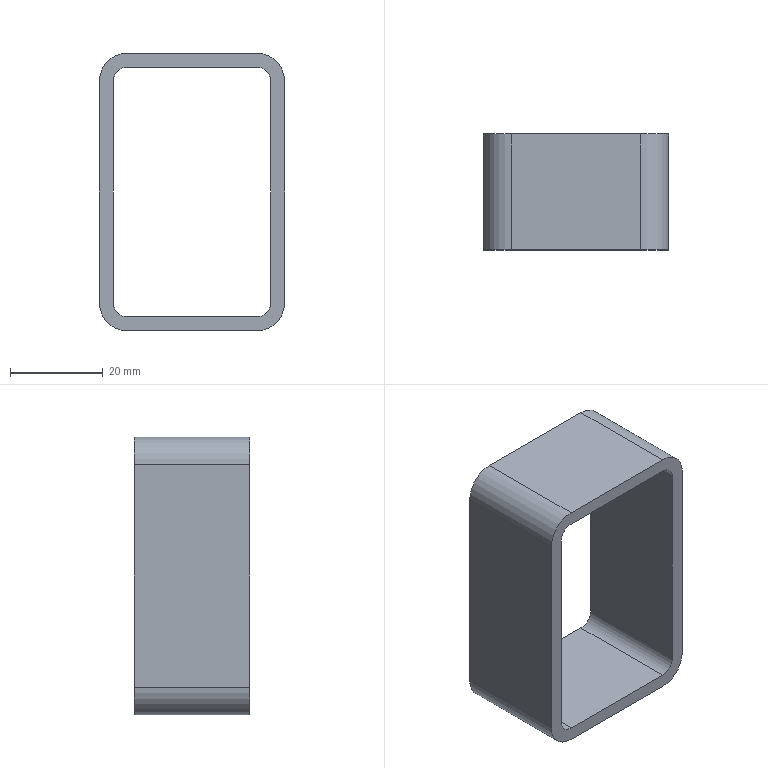Part | SolidWorks | features WeldMemberFeat 1, WeldmentFeature 1 | 1 solid | 18 faces | box 40 x 25 x 60 mm | volume 13521 mm3 | plane 10 | cylinder 8 | commonest cylinder face diameters 6 x4 12 x4
STEP:
#1=CARTESIAN_POINT('',(-20.,0.,24.));
#2=VERTEX_POINT('',#1);
#3=CARTESIAN_POINT('',(-14.,0.,30.));
#4=VERTEX_POINT('',#3);
#5=CARTESIAN_POINT('',(-14.,0.,24.));
#6=DIRECTION('',(0.,1.,0.));
#7=DIRECTION('',(0.,0.,1.));
#8=AXIS2_PLACEMENT_3D('',#5,#6,#7);
#9=CIRCLE('',#8,6.);
#10=EDGE_CURVE('',#2,#4,#9,.T.);
#11=ORIENTED_EDGE('',*,*,#10,.T.);
#12=CARTESIAN_POINT('',(-14.,25.,30.));
#13=VERTEX_POINT('',#12);
#14=CARTESIAN_POINT('',(-14.,25.,30.));
#15=DIRECTION('',(0.,-1.,0.));
#16=VECTOR('',#15,1000.);
#17=LINE('',#14,#16);
#18=EDGE_CURVE('',#13,#4,#17,.T.);
#19=ORIENTED_EDGE('',*,*,#18,.F.);
#20=CARTESIAN_POINT('',(-20.,25.,24.));
#21=VERTEX_POINT('',#20);
#22=CARTESIAN_POINT('',(-14.,25.,24.));
#23=DIRECTION('',(0.,1.,0.));
#24=DIRECTION('',(0.,0.,1.));
#25=AXIS2_PLACEMENT_3D('',#22,#23,#24);
#26=CIRCLE('',#25,6.);
#27=EDGE_CURVE('',#21,#13,#26,.T.);
#28=ORIENTED_EDGE('',*,*,#27,.F.);
#29=CARTESIAN_POINT('',(-20.,25.,24.));
#30=DIRECTION('',(0.,-1.,0.));
#31=VECTOR('',#30,1000.);
#32=LINE('',#29,#31);
#33=EDGE_CURVE('',#21,#2,#32,.T.);
#34=ORIENTED_EDGE('',*,*,#33,.T.);
#35=EDGE_LOOP('',(#11,#19,#28,#34));
#36=FACE_OUTER_BOUND('',#35,.T.);
#37=CARTESIAN_POINT('',(-14.,25.,24.));
#38=DIRECTION('',(0.,-1.,0.));
#39=DIRECTION('',(0.,0.,-1.));
#40=AXIS2_PLACEMENT_3D('',#37,#38,#39);
#41=CYLINDRICAL_SURFACE('',#40,6.);
#42=ADVANCED_FACE('',(#36),#41,.T.);
#43=CARTESIAN_POINT('',(14.,0.,30.));
#44=VERTEX_POINT('',#43);
#45=CARTESIAN_POINT('',(-14.,0.,30.));
#46=DIRECTION('',(1.,0.,0.));
#47=VECTOR('',#46,1000.);
#48=LINE('',#45,#47);
#49=EDGE_CURVE('',#4,#44,#48,.T.);
#50=ORIENTED_EDGE('',*,*,#49,.T.);
#51=CARTESIAN_POINT('',(14.,25.,30.));
#52=VERTEX_POINT('',#51);
#53=CARTESIAN_POINT('',(14.,25.,30.));
#54=DIRECTION('',(0.,-1.,0.));
#55=VECTOR('',#54,1000.);
#56=LINE('',#53,#55);
#57=EDGE_CURVE('',#52,#44,#56,.T.);
#58=ORIENTED_EDGE('',*,*,#57,.F.);
#59=CARTESIAN_POINT('',(-14.,25.,30.));
#60=DIRECTION('',(1.,0.,0.));
#61=VECTOR('',#60,1000.);
#62=LINE('',#59,#61);
#63=EDGE_CURVE('',#13,#52,#62,.T.);
#64=ORIENTED_EDGE('',*,*,#63,.F.);
#65=ORIENTED_EDGE('',*,*,#18,.T.);
#66=EDGE_LOOP('',(#50,#58,#64,#65));
#67=FACE_OUTER_BOUND('',#66,.T.);
#68=CARTESIAN_POINT('',(-14.,25.,30.));
#69=DIRECTION('',(0.,0.,-1.));
#70=DIRECTION('',(-1.,0.,0.));
#71=AXIS2_PLACEMENT_3D('',#68,#69,#70);
#72=PLANE('',#71);
#73=ADVANCED_FACE('',(#67),#72,.F.);
#74=CARTESIAN_POINT('',(20.,0.,24.));
#75=VERTEX_POINT('',#74);
#76=CARTESIAN_POINT('',(14.,0.,24.));
#77=DIRECTION('',(0.,1.,0.));
#78=DIRECTION('',(0.,0.,1.));
#79=AXIS2_PLACEMENT_3D('',#76,#77,#78);
#80=CIRCLE('',#79,6.);
#81=EDGE_CURVE('',#44,#75,#80,.T.);
#82=ORIENTED_EDGE('',*,*,#81,.T.);
#83=CARTESIAN_POINT('',(20.,25.,24.));
#84=VERTEX_POINT('',#83);
#85=CARTESIAN_POINT('',(20.,25.,24.));
#86=DIRECTION('',(0.,-1.,0.));
#87=VECTOR('',#86,1000.);
#88=LINE('',#85,#87);
#89=EDGE_CURVE('',#84,#75,#88,.T.);
#90=ORIENTED_EDGE('',*,*,#89,.F.);
#91=CARTESIAN_POINT('',(14.,25.,24.));
#92=DIRECTION('',(0.,1.,0.));
#93=DIRECTION('',(0.,0.,1.));
#94=AXIS2_PLACEMENT_3D('',#91,#92,#93);
#95=CIRCLE('',#94,6.);
#96=EDGE_CURVE('',#52,#84,#95,.T.);
#97=ORIENTED_EDGE('',*,*,#96,.F.);
#98=ORIENTED_EDGE('',*,*,#57,.T.);
#99=EDGE_LOOP('',(#82,#90,#97,#98));
#100=FACE_OUTER_BOUND('',#99,.T.);
#101=CARTESIAN_POINT('',(14.,25.,24.));
#102=DIRECTION('',(0.,-1.,0.));
#103=DIRECTION('',(0.,0.,-1.));
#104=AXIS2_PLACEMENT_3D('',#101,#102,#103);
#105=CYLINDRICAL_SURFACE('',#104,6.);
#106=ADVANCED_FACE('',(#100),#105,.T.);
#107=CARTESIAN_POINT('',(20.,0.,-24.));
#108=VERTEX_POINT('',#107);
#109=CARTESIAN_POINT('',(20.,0.,-24.));
#110=DIRECTION('',(0.,0.,-1.));
#111=VECTOR('',#110,1000.);
#112=LINE('',#109,#111);
#113=EDGE_CURVE('',#75,#108,#112,.T.);
#114=ORIENTED_EDGE('',*,*,#113,.T.);
#115=CARTESIAN_POINT('',(20.,25.,-24.));
#116=VERTEX_POINT('',#115);
#117=CARTESIAN_POINT('',(20.,25.,-24.));
#118=DIRECTION('',(0.,-1.,0.));
#119=VECTOR('',#118,1000.);
#120=LINE('',#117,#119);
#121=EDGE_CURVE('',#116,#108,#120,.T.);
#122=ORIENTED_EDGE('',*,*,#121,.F.);
#123=CARTESIAN_POINT('',(20.,25.,-24.));
#124=DIRECTION('',(0.,0.,-1.));
#125=VECTOR('',#124,1000.);
#126=LINE('',#123,#125);
#127=EDGE_CURVE('',#84,#116,#126,.T.);
#128=ORIENTED_EDGE('',*,*,#127,.F.);
#129=ORIENTED_EDGE('',*,*,#89,.T.);
#130=EDGE_LOOP('',(#114,#122,#128,#129));
#131=FACE_OUTER_BOUND('',#130,.T.);
#132=CARTESIAN_POINT('',(20.,25.,-24.));
#133=DIRECTION('',(-1.,0.,0.));
#134=DIRECTION('',(0.,0.,1.));
#135=AXIS2_PLACEMENT_3D('',#132,#133,#134);
#136=PLANE('',#135);
#137=ADVANCED_FACE('',(#131),#136,.F.);
#138=CARTESIAN_POINT('',(14.,0.,-30.));
#139=VERTEX_POINT('',#138);
#140=CARTESIAN_POINT('',(14.,0.,-24.));
#141=DIRECTION('',(0.,1.,0.));
#142=DIRECTION('',(0.,0.,1.));
#143=AXIS2_PLACEMENT_3D('',#140,#141,#142);
#144=CIRCLE('',#143,6.);
#145=EDGE_CURVE('',#108,#139,#144,.T.);
#146=ORIENTED_EDGE('',*,*,#145,.T.);
#147=CARTESIAN_POINT('',(14.,25.,-30.));
#148=VERTEX_POINT('',#147);
#149=CARTESIAN_POINT('',(14.,25.,-30.));
#150=DIRECTION('',(0.,-1.,0.));
#151=VECTOR('',#150,1000.);
#152=LINE('',#149,#151);
#153=EDGE_CURVE('',#148,#139,#152,.T.);
#154=ORIENTED_EDGE('',*,*,#153,.F.);
#155=CARTESIAN_POINT('',(14.,25.,-24.));
#156=DIRECTION('',(0.,1.,0.));
#157=DIRECTION('',(0.,0.,1.));
#158=AXIS2_PLACEMENT_3D('',#155,#156,#157);
#159=CIRCLE('',#158,6.);
#160=EDGE_CURVE('',#116,#148,#159,.T.);
#161=ORIENTED_EDGE('',*,*,#160,.F.);
#162=ORIENTED_EDGE('',*,*,#121,.T.);
#163=EDGE_LOOP('',(#146,#154,#161,#162));
#164=FACE_OUTER_BOUND('',#163,.T.);
#165=CARTESIAN_POINT('',(14.,25.,-24.));
#166=DIRECTION('',(0.,-1.,0.));
#167=DIRECTION('',(0.,0.,-1.));
#168=AXIS2_PLACEMENT_3D('',#165,#166,#167);
#169=CYLINDRICAL_SURFACE('',#168,6.);
#170=ADVANCED_FACE('',(#164),#169,.T.);
#171=CARTESIAN_POINT('',(-14.,0.,-30.));
#172=VERTEX_POINT('',#171);
#173=CARTESIAN_POINT('',(14.,0.,-30.));
#174=DIRECTION('',(-1.,0.,0.));
#175=VECTOR('',#174,1000.);
#176=LINE('',#173,#175);
#177=EDGE_CURVE('',#139,#172,#176,.T.);
#178=ORIENTED_EDGE('',*,*,#177,.T.);
#179=CARTESIAN_POINT('',(-14.,25.,-30.));
#180=VERTEX_POINT('',#179);
#181=CARTESIAN_POINT('',(-14.,25.,-30.));
#182=DIRECTION('',(0.,-1.,0.));
#183=VECTOR('',#182,1000.);
#184=LINE('',#181,#183);
#185=EDGE_CURVE('',#180,#172,#184,.T.);
#186=ORIENTED_EDGE('',*,*,#185,.F.);
#187=CARTESIAN_POINT('',(14.,25.,-30.));
#188=DIRECTION('',(-1.,0.,0.));
#189=VECTOR('',#188,1000.);
#190=LINE('',#187,#189);
#191=EDGE_CURVE('',#148,#180,#190,.T.);
#192=ORIENTED_EDGE('',*,*,#191,.F.);
#193=ORIENTED_EDGE('',*,*,#153,.T.);
#194=EDGE_LOOP('',(#178,#186,#192,#193));
#195=FACE_OUTER_BOUND('',#194,.T.);
#196=CARTESIAN_POINT('',(14.,25.,-30.));
#197=DIRECTION('',(0.,0.,1.));
#198=DIRECTION('',(1.,0.,0.));
#199=AXIS2_PLACEMENT_3D('',#196,#197,#198);
#200=PLANE('',#199);
#201=ADVANCED_FACE('',(#195),#200,.F.);
#202=CARTESIAN_POINT('',(-20.,0.,-24.));
#203=VERTEX_POINT('',#202);
#204=CARTESIAN_POINT('',(-14.,0.,-24.));
#205=DIRECTION('',(0.,1.,0.));
#206=DIRECTION('',(0.,0.,1.));
#207=AXIS2_PLACEMENT_3D('',#204,#205,#206);
#208=CIRCLE('',#207,6.);
#209=EDGE_CURVE('',#172,#203,#208,.T.);
#210=ORIENTED_EDGE('',*,*,#209,.T.);
#211=CARTESIAN_POINT('',(-20.,25.,-24.));
#212=VERTEX_POINT('',#211);
#213=CARTESIAN_POINT('',(-20.,25.,-24.));
#214=DIRECTION('',(0.,-1.,0.));
#215=VECTOR('',#214,1000.);
#216=LINE('',#213,#215);
#217=EDGE_CURVE('',#212,#203,#216,.T.);
#218=ORIENTED_EDGE('',*,*,#217,.F.);
#219=CARTESIAN_POINT('',(-14.,25.,-24.));
#220=DIRECTION('',(0.,1.,0.));
#221=DIRECTION('',(0.,0.,1.));
#222=AXIS2_PLACEMENT_3D('',#219,#220,#221);
#223=CIRCLE('',#222,6.);
#224=EDGE_CURVE('',#180,#212,#223,.T.);
#225=ORIENTED_EDGE('',*,*,#224,.F.);
#226=ORIENTED_EDGE('',*,*,#185,.T.);
#227=EDGE_LOOP('',(#210,#218,#225,#226));
#228=FACE_OUTER_BOUND('',#227,.T.);
#229=CARTESIAN_POINT('',(-14.,25.,-24.));
#230=DIRECTION('',(0.,-1.,0.));
#231=DIRECTION('',(0.,0.,-1.));
#232=AXIS2_PLACEMENT_3D('',#229,#230,#231);
#233=CYLINDRICAL_SURFACE('',#232,6.);
#234=ADVANCED_FACE('',(#228),#233,.T.);
#235=CARTESIAN_POINT('',(14.,0.,27.));
#236=VERTEX_POINT('',#235);
#237=CARTESIAN_POINT('',(17.,0.,24.));
#238=VERTEX_POINT('',#237);
#239=CARTESIAN_POINT('',(14.,0.,24.));
#240=DIRECTION('',(0.,1.,0.));
#241=DIRECTION('',(0.,0.,1.));
#242=AXIS2_PLACEMENT_3D('',#239,#240,#241);
#243=CIRCLE('',#242,3.);
#244=EDGE_CURVE('',#236,#238,#243,.T.);
#245=ORIENTED_EDGE('',*,*,#244,.F.);
#246=CARTESIAN_POINT('',(14.,25.,27.));
#247=VERTEX_POINT('',#246);
#248=CARTESIAN_POINT('',(14.,25.,27.));
#249=DIRECTION('',(0.,-1.,0.));
#250=VECTOR('',#249,1000.);
#251=LINE('',#248,#250);
#252=EDGE_CURVE('',#247,#236,#251,.T.);
#253=ORIENTED_EDGE('',*,*,#252,.F.);
#254=CARTESIAN_POINT('',(17.,25.,24.));
#255=VERTEX_POINT('',#254);
#256=CARTESIAN_POINT('',(14.,25.,24.));
#257=DIRECTION('',(0.,1.,0.));
#258=DIRECTION('',(0.,0.,1.));
#259=AXIS2_PLACEMENT_3D('',#256,#257,#258);
#260=CIRCLE('',#259,3.);
#261=EDGE_CURVE('',#247,#255,#260,.T.);
#262=ORIENTED_EDGE('',*,*,#261,.T.);
#263=CARTESIAN_POINT('',(17.,25.,24.));
#264=DIRECTION('',(0.,-1.,0.));
#265=VECTOR('',#264,1000.);
#266=LINE('',#263,#265);
#267=EDGE_CURVE('',#255,#238,#266,.T.);
#268=ORIENTED_EDGE('',*,*,#267,.T.);
#269=EDGE_LOOP('',(#245,#253,#262,#268));
#270=FACE_OUTER_BOUND('',#269,.T.);
#271=CARTESIAN_POINT('',(14.,25.,24.));
#272=DIRECTION('',(0.,-1.,0.));
#273=DIRECTION('',(0.,0.,-1.));
#274=AXIS2_PLACEMENT_3D('',#271,#272,#273);
#275=CYLINDRICAL_SURFACE('',#274,3.);
#276=ADVANCED_FACE('',(#270),#275,.F.);
#277=CARTESIAN_POINT('',(-14.,0.,27.));
#278=VERTEX_POINT('',#277);
#279=CARTESIAN_POINT('',(-14.,0.,27.));
#280=DIRECTION('',(1.,0.,0.));
#281=VECTOR('',#280,1000.);
#282=LINE('',#279,#281);
#283=EDGE_CURVE('',#278,#236,#282,.T.);
#284=ORIENTED_EDGE('',*,*,#283,.F.);
#285=CARTESIAN_POINT('',(-14.,25.,27.));
#286=VERTEX_POINT('',#285);
#287=CARTESIAN_POINT('',(-14.,25.,27.));
#288=DIRECTION('',(0.,-1.,0.));
#289=VECTOR('',#288,1000.);
#290=LINE('',#287,#289);
#291=EDGE_CURVE('',#286,#278,#290,.T.);
#292=ORIENTED_EDGE('',*,*,#291,.F.);
#293=CARTESIAN_POINT('',(-14.,25.,27.));
#294=DIRECTION('',(1.,0.,0.));
#295=VECTOR('',#294,1000.);
#296=LINE('',#293,#295);
#297=EDGE_CURVE('',#286,#247,#296,.T.);
#298=ORIENTED_EDGE('',*,*,#297,.T.);
#299=ORIENTED_EDGE('',*,*,#252,.T.);
#300=EDGE_LOOP('',(#284,#292,#298,#299));
#301=FACE_OUTER_BOUND('',#300,.T.);
#302=CARTESIAN_POINT('',(-14.,25.,27.));
#303=DIRECTION('',(0.,0.,-1.));
#304=DIRECTION('',(-1.,0.,0.));
#305=AXIS2_PLACEMENT_3D('',#302,#303,#304);
#306=PLANE('',#305);
#307=ADVANCED_FACE('',(#301),#306,.T.);
#308=CARTESIAN_POINT('',(-17.,0.,24.));
#309=VERTEX_POINT('',#308);
#310=CARTESIAN_POINT('',(-14.,0.,24.));
#311=DIRECTION('',(0.,1.,0.));
#312=DIRECTION('',(0.,0.,1.));
#313=AXIS2_PLACEMENT_3D('',#310,#311,#312);
#314=CIRCLE('',#313,3.);
#315=EDGE_CURVE('',#309,#278,#314,.T.);
#316=ORIENTED_EDGE('',*,*,#315,.F.);
#317=CARTESIAN_POINT('',(-17.,25.,24.));
#318=VERTEX_POINT('',#317);
#319=CARTESIAN_POINT('',(-17.,25.,24.));
#320=DIRECTION('',(0.,-1.,0.));
#321=VECTOR('',#320,1000.);
#322=LINE('',#319,#321);
#323=EDGE_CURVE('',#318,#309,#322,.T.);
#324=ORIENTED_EDGE('',*,*,#323,.F.);
#325=CARTESIAN_POINT('',(-14.,25.,24.));
#326=DIRECTION('',(0.,1.,0.));
#327=DIRECTION('',(0.,0.,1.));
#328=AXIS2_PLACEMENT_3D('',#325,#326,#327);
#329=CIRCLE('',#328,3.);
#330=EDGE_CURVE('',#318,#286,#329,.T.);
#331=ORIENTED_EDGE('',*,*,#330,.T.);
#332=ORIENTED_EDGE('',*,*,#291,.T.);
#333=EDGE_LOOP('',(#316,#324,#331,#332));
#334=FACE_OUTER_BOUND('',#333,.T.);
#335=CARTESIAN_POINT('',(-14.,25.,24.));
#336=DIRECTION('',(0.,-1.,0.));
#337=DIRECTION('',(0.,0.,-1.));
#338=AXIS2_PLACEMENT_3D('',#335,#336,#337);
#339=CYLINDRICAL_SURFACE('',#338,3.);
#340=ADVANCED_FACE('',(#334),#339,.F.);
#341=CARTESIAN_POINT('',(-17.,0.,-24.));
#342=VERTEX_POINT('',#341);
#343=CARTESIAN_POINT('',(-17.,0.,24.));
#344=DIRECTION('',(0.,0.,1.));
#345=VECTOR('',#344,1000.);
#346=LINE('',#343,#345);
#347=EDGE_CURVE('',#342,#309,#346,.T.);
#348=ORIENTED_EDGE('',*,*,#347,.F.);
#349=CARTESIAN_POINT('',(-17.,25.,-24.));
#350=VERTEX_POINT('',#349);
#351=CARTESIAN_POINT('',(-17.,25.,-24.));
#352=DIRECTION('',(0.,-1.,0.));
#353=VECTOR('',#352,1000.);
#354=LINE('',#351,#353);
#355=EDGE_CURVE('',#350,#342,#354,.T.);
#356=ORIENTED_EDGE('',*,*,#355,.F.);
#357=CARTESIAN_POINT('',(-17.,25.,24.));
#358=DIRECTION('',(0.,0.,1.));
#359=VECTOR('',#358,1000.);
#360=LINE('',#357,#359);
#361=EDGE_CURVE('',#350,#318,#360,.T.);
#362=ORIENTED_EDGE('',*,*,#361,.T.);
#363=ORIENTED_EDGE('',*,*,#323,.T.);
#364=EDGE_LOOP('',(#348,#356,#362,#363));
#365=FACE_OUTER_BOUND('',#364,.T.);
#366=CARTESIAN_POINT('',(-17.,25.,24.));
#367=DIRECTION('',(1.,0.,0.));
#368=DIRECTION('',(0.,0.,-1.));
#369=AXIS2_PLACEMENT_3D('',#366,#367,#368);
#370=PLANE('',#369);
#371=ADVANCED_FACE('',(#365),#370,.T.);
#372=CARTESIAN_POINT('',(-14.,0.,-27.));
#373=VERTEX_POINT('',#372);
#374=CARTESIAN_POINT('',(-14.,0.,-24.));
#375=DIRECTION('',(0.,1.,0.));
#376=DIRECTION('',(0.,0.,1.));
#377=AXIS2_PLACEMENT_3D('',#374,#375,#376);
#378=CIRCLE('',#377,3.);
#379=EDGE_CURVE('',#373,#342,#378,.T.);
#380=ORIENTED_EDGE('',*,*,#379,.F.);
#381=CARTESIAN_POINT('',(-14.,25.,-27.));
#382=VERTEX_POINT('',#381);
#383=CARTESIAN_POINT('',(-14.,25.,-27.));
#384=DIRECTION('',(0.,-1.,0.));
#385=VECTOR('',#384,1000.);
#386=LINE('',#383,#385);
#387=EDGE_CURVE('',#382,#373,#386,.T.);
#388=ORIENTED_EDGE('',*,*,#387,.F.);
#389=CARTESIAN_POINT('',(-14.,25.,-24.));
#390=DIRECTION('',(0.,1.,0.));
#391=DIRECTION('',(0.,0.,1.));
#392=AXIS2_PLACEMENT_3D('',#389,#390,#391);
#393=CIRCLE('',#392,3.);
#394=EDGE_CURVE('',#382,#350,#393,.T.);
#395=ORIENTED_EDGE('',*,*,#394,.T.);
#396=ORIENTED_EDGE('',*,*,#355,.T.);
#397=EDGE_LOOP('',(#380,#388,#395,#396));
#398=FACE_OUTER_BOUND('',#397,.T.);
#399=CARTESIAN_POINT('',(-14.,25.,-24.));
#400=DIRECTION('',(0.,-1.,0.));
#401=DIRECTION('',(0.,0.,-1.));
#402=AXIS2_PLACEMENT_3D('',#399,#400,#401);
#403=CYLINDRICAL_SURFACE('',#402,3.);
#404=ADVANCED_FACE('',(#398),#403,.F.);
#405=CARTESIAN_POINT('',(14.,0.,-27.));
#406=VERTEX_POINT('',#405);
#407=CARTESIAN_POINT('',(14.,0.,-27.));
#408=DIRECTION('',(-1.,0.,0.));
#409=VECTOR('',#408,1000.);
#410=LINE('',#407,#409);
#411=EDGE_CURVE('',#406,#373,#410,.T.);
#412=ORIENTED_EDGE('',*,*,#411,.F.);
#413=CARTESIAN_POINT('',(14.,25.,-27.));
#414=VERTEX_POINT('',#413);
#415=CARTESIAN_POINT('',(14.,25.,-27.));
#416=DIRECTION('',(0.,-1.,0.));
#417=VECTOR('',#416,1000.);
#418=LINE('',#415,#417);
#419=EDGE_CURVE('',#414,#406,#418,.T.);
#420=ORIENTED_EDGE('',*,*,#419,.F.);
#421=CARTESIAN_POINT('',(14.,25.,-27.));
#422=DIRECTION('',(-1.,0.,0.));
#423=VECTOR('',#422,1000.);
#424=LINE('',#421,#423);
#425=EDGE_CURVE('',#414,#382,#424,.T.);
#426=ORIENTED_EDGE('',*,*,#425,.T.);
#427=ORIENTED_EDGE('',*,*,#387,.T.);
#428=EDGE_LOOP('',(#412,#420,#426,#427));
#429=FACE_OUTER_BOUND('',#428,.T.);
#430=CARTESIAN_POINT('',(14.,25.,-27.));
#431=DIRECTION('',(0.,0.,1.));
#432=DIRECTION('',(1.,0.,0.));
#433=AXIS2_PLACEMENT_3D('',#430,#431,#432);
#434=PLANE('',#433);
#435=ADVANCED_FACE('',(#429),#434,.T.);
#436=CARTESIAN_POINT('',(17.,0.,-24.));
#437=VERTEX_POINT('',#436);
#438=CARTESIAN_POINT('',(14.,0.,-24.));
#439=DIRECTION('',(0.,1.,0.));
#440=DIRECTION('',(0.,0.,1.));
#441=AXIS2_PLACEMENT_3D('',#438,#439,#440);
#442=CIRCLE('',#441,3.);
#443=EDGE_CURVE('',#437,#406,#442,.T.);
#444=ORIENTED_EDGE('',*,*,#443,.F.);
#445=CARTESIAN_POINT('',(17.,25.,-24.));
#446=VERTEX_POINT('',#445);
#447=CARTESIAN_POINT('',(17.,25.,-24.));
#448=DIRECTION('',(0.,-1.,0.));
#449=VECTOR('',#448,1000.);
#450=LINE('',#447,#449);
#451=EDGE_CURVE('',#446,#437,#450,.T.);
#452=ORIENTED_EDGE('',*,*,#451,.F.);
#453=CARTESIAN_POINT('',(14.,25.,-24.));
#454=DIRECTION('',(0.,1.,0.));
#455=DIRECTION('',(0.,0.,1.));
#456=AXIS2_PLACEMENT_3D('',#453,#454,#455);
#457=CIRCLE('',#456,3.);
#458=EDGE_CURVE('',#446,#414,#457,.T.);
#459=ORIENTED_EDGE('',*,*,#458,.T.);
#460=ORIENTED_EDGE('',*,*,#419,.T.);
#461=EDGE_LOOP('',(#444,#452,#459,#460));
#462=FACE_OUTER_BOUND('',#461,.T.);
#463=CARTESIAN_POINT('',(14.,25.,-24.));
#464=DIRECTION('',(0.,-1.,0.));
#465=DIRECTION('',(0.,0.,-1.));
#466=AXIS2_PLACEMENT_3D('',#463,#464,#465);
#467=CYLINDRICAL_SURFACE('',#466,3.);
#468=ADVANCED_FACE('',(#462),#467,.F.);
#469=CARTESIAN_POINT('',(17.,0.,-24.));
#470=DIRECTION('',(0.,0.,-1.));
#471=VECTOR('',#470,1000.);
#472=LINE('',#469,#471);
#473=EDGE_CURVE('',#238,#437,#472,.T.);
#474=ORIENTED_EDGE('',*,*,#473,.F.);
#475=ORIENTED_EDGE('',*,*,#267,.F.);
#476=CARTESIAN_POINT('',(17.,25.,-24.));
#477=DIRECTION('',(0.,0.,-1.));
#478=VECTOR('',#477,1000.);
#479=LINE('',#476,#478);
#480=EDGE_CURVE('',#255,#446,#479,.T.);
#481=ORIENTED_EDGE('',*,*,#480,.T.);
#482=ORIENTED_EDGE('',*,*,#451,.T.);
#483=EDGE_LOOP('',(#474,#475,#481,#482));
#484=FACE_OUTER_BOUND('',#483,.T.);
#485=CARTESIAN_POINT('',(17.,25.,-24.));
#486=DIRECTION('',(-1.,0.,0.));
#487=DIRECTION('',(0.,0.,1.));
#488=AXIS2_PLACEMENT_3D('',#485,#486,#487);
#489=PLANE('',#488);
#490=ADVANCED_FACE('',(#484),#489,.T.);
#491=CARTESIAN_POINT('',(-20.,0.,24.));
#492=DIRECTION('',(0.,0.,1.));
#493=VECTOR('',#492,1000.);
#494=LINE('',#491,#493);
#495=EDGE_CURVE('',#203,#2,#494,.T.);
#496=ORIENTED_EDGE('',*,*,#495,.T.);
#497=ORIENTED_EDGE('',*,*,#33,.F.);
#498=CARTESIAN_POINT('',(-20.,25.,24.));
#499=DIRECTION('',(0.,0.,1.));
#500=VECTOR('',#499,1000.);
#501=LINE('',#498,#500);
#502=EDGE_CURVE('',#212,#21,#501,.T.);
#503=ORIENTED_EDGE('',*,*,#502,.F.);
#504=ORIENTED_EDGE('',*,*,#217,.T.);
#505=EDGE_LOOP('',(#496,#497,#503,#504));
#506=FACE_OUTER_BOUND('',#505,.T.);
#507=CARTESIAN_POINT('',(-20.,25.,24.));
#508=DIRECTION('',(1.,0.,0.));
#509=DIRECTION('',(0.,0.,-1.));
#510=AXIS2_PLACEMENT_3D('',#507,#508,#509);
#511=PLANE('',#510);
#512=ADVANCED_FACE('',(#506),#511,.F.);
#513=ORIENTED_EDGE('',*,*,#261,.F.);
#514=ORIENTED_EDGE('',*,*,#297,.F.);
#515=ORIENTED_EDGE('',*,*,#330,.F.);
#516=ORIENTED_EDGE('',*,*,#361,.F.);
#517=ORIENTED_EDGE('',*,*,#394,.F.);
#518=ORIENTED_EDGE('',*,*,#425,.F.);
#519=ORIENTED_EDGE('',*,*,#458,.F.);
#520=ORIENTED_EDGE('',*,*,#480,.F.);
#521=EDGE_LOOP('',(#513,#514,#515,#516,#517,#518,#519,#520));
#522=FACE_BOUND('',#521,.T.);
#523=ORIENTED_EDGE('',*,*,#27,.T.);
#524=ORIENTED_EDGE('',*,*,#63,.T.);
#525=ORIENTED_EDGE('',*,*,#96,.T.);
#526=ORIENTED_EDGE('',*,*,#127,.T.);
#527=ORIENTED_EDGE('',*,*,#160,.T.);
#528=ORIENTED_EDGE('',*,*,#191,.T.);
#529=ORIENTED_EDGE('',*,*,#224,.T.);
#530=ORIENTED_EDGE('',*,*,#502,.T.);
#531=EDGE_LOOP('',(#523,#524,#525,#526,#527,#528,#529,#530));
#532=FACE_OUTER_BOUND('',#531,.T.);
#533=CARTESIAN_POINT('',(-14.,25.,24.));
#534=DIRECTION('',(0.,1.,0.));
#535=DIRECTION('',(0.,0.,1.));
#536=AXIS2_PLACEMENT_3D('',#533,#534,#535);
#537=PLANE('',#536);
#538=ADVANCED_FACE('',(#522,#532),#537,.T.);
#539=ORIENTED_EDGE('',*,*,#244,.T.);
#540=ORIENTED_EDGE('',*,*,#473,.T.);
#541=ORIENTED_EDGE('',*,*,#443,.T.);
#542=ORIENTED_EDGE('',*,*,#411,.T.);
#543=ORIENTED_EDGE('',*,*,#379,.T.);
#544=ORIENTED_EDGE('',*,*,#347,.T.);
#545=ORIENTED_EDGE('',*,*,#315,.T.);
#546=ORIENTED_EDGE('',*,*,#283,.T.);
#547=EDGE_LOOP('',(#539,#540,#541,#542,#543,#544,#545,#546));
#548=FACE_BOUND('',#547,.T.);
#549=ORIENTED_EDGE('',*,*,#10,.F.);
#550=ORIENTED_EDGE('',*,*,#495,.F.);
#551=ORIENTED_EDGE('',*,*,#209,.F.);
#552=ORIENTED_EDGE('',*,*,#177,.F.);
#553=ORIENTED_EDGE('',*,*,#145,.F.);
#554=ORIENTED_EDGE('',*,*,#113,.F.);
#555=ORIENTED_EDGE('',*,*,#81,.F.);
#556=ORIENTED_EDGE('',*,*,#49,.F.);
#557=EDGE_LOOP('',(#549,#550,#551,#552,#553,#554,#555,#556));
#558=FACE_OUTER_BOUND('',#557,.T.);
#559=CARTESIAN_POINT('',(-14.,0.,24.));
#560=DIRECTION('',(0.,1.,0.));
#561=DIRECTION('',(0.,0.,1.));
#562=AXIS2_PLACEMENT_3D('',#559,#560,#561);
#563=PLANE('',#562);
#564=ADVANCED_FACE('',(#548,#558),#563,.F.);
#565=CLOSED_SHELL('',(#42,#73,#106,#137,#170,#201,#234,#276,#307,#340,#371,#404,#435,#468,#490,#512,#538,#564));
#566=MANIFOLD_SOLID_BREP('',#565);
#567=CARTESIAN_POINT('',(0.,0.,0.));
#568=DIRECTION('',(0.,0.,1.));
#569=DIRECTION('',(1.,0.,0.));
#570=AXIS2_PLACEMENT_3D('',#567,#568,#569);
#571=(LENGTH_UNIT()NAMED_UNIT(*)SI_UNIT(.MILLI.,.METRE.));
#572=UNCERTAINTY_MEASURE_WITH_UNIT(LENGTH_MEASURE(0.00001),#571,'','');
#573=(NAMED_UNIT(*)PLANE_ANGLE_UNIT()SI_UNIT($,.RADIAN.));
#574=(NAMED_UNIT(*)SI_UNIT($,.STERADIAN.)SOLID_ANGLE_UNIT());
#575=(GEOMETRIC_REPRESENTATION_CONTEXT(3)GLOBAL_UNCERTAINTY_ASSIGNED_CONTEXT((#572))GLOBAL_UNIT_ASSIGNED_CONTEXT((#571,#573,#574))REPRESENTATION_CONTEXT('',''));
#576=ADVANCED_BREP_SHAPE_REPRESENTATION('',(#566,#570),#575);